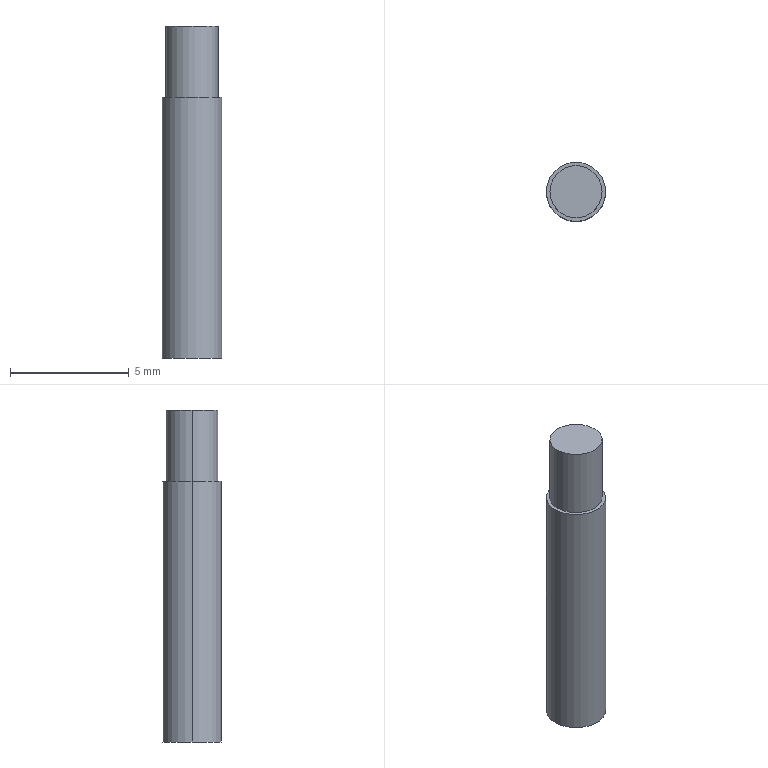Part | SolidWorks | features Extrusion 1, ICE 1 | 1 solid | 7 faces | box 2.5 x 2.5 x 14 mm | volume 65.4 mm3 | cylinder 4 | plane 3 | commonest cylinder face diameters 2.2 x2 2.5 x2
STEP:
#1=CARTESIAN_POINT('',(1.1,0.,14.));
#2=VERTEX_POINT('',#1);
#3=CARTESIAN_POINT('',(-1.1,0.,14.));
#4=VERTEX_POINT('',#3);
#5=CARTESIAN_POINT('',(0.,0.,14.));
#6=DIRECTION('',(0.,0.,1.));
#7=DIRECTION('',(1.,0.,0.));
#8=AXIS2_PLACEMENT_3D('',#5,#6,#7);
#9=CIRCLE('',#8,1.1);
#10=EDGE_CURVE('',#2,#4,#9,.T.);
#11=ORIENTED_EDGE('',*,*,#10,.F.);
#12=CARTESIAN_POINT('',(1.1,0.,11.));
#13=VERTEX_POINT('',#12);
#14=CARTESIAN_POINT('',(1.1,0.,14.));
#15=DIRECTION('',(0.,0.,-1.));
#16=VECTOR('',#15,1000.);
#17=LINE('',#14,#16);
#18=EDGE_CURVE('',#2,#13,#17,.T.);
#19=ORIENTED_EDGE('',*,*,#18,.T.);
#20=CARTESIAN_POINT('',(-1.1,0.,11.));
#21=VERTEX_POINT('',#20);
#22=CARTESIAN_POINT('',(0.,0.,11.));
#23=DIRECTION('',(0.,0.,1.));
#24=DIRECTION('',(1.,0.,0.));
#25=AXIS2_PLACEMENT_3D('',#22,#23,#24);
#26=CIRCLE('',#25,1.1);
#27=EDGE_CURVE('',#13,#21,#26,.T.);
#28=ORIENTED_EDGE('',*,*,#27,.T.);
#29=CARTESIAN_POINT('',(-1.1,0.,14.));
#30=DIRECTION('',(0.,0.,-1.));
#31=VECTOR('',#30,1000.);
#32=LINE('',#29,#31);
#33=EDGE_CURVE('',#4,#21,#32,.T.);
#34=ORIENTED_EDGE('',*,*,#33,.F.);
#35=EDGE_LOOP('',(#11,#19,#28,#34));
#36=FACE_OUTER_BOUND('',#35,.T.);
#37=CARTESIAN_POINT('',(0.,0.,14.));
#38=DIRECTION('',(0.,0.,-1.));
#39=DIRECTION('',(-1.,0.,0.));
#40=AXIS2_PLACEMENT_3D('',#37,#38,#39);
#41=CYLINDRICAL_SURFACE('',#40,1.1);
#42=ADVANCED_FACE('',(#36),#41,.T.);
#43=CARTESIAN_POINT('',(1.25,0.,11.));
#44=VERTEX_POINT('',#43);
#45=CARTESIAN_POINT('',(-1.25,0.,11.));
#46=VERTEX_POINT('',#45);
#47=CARTESIAN_POINT('',(0.,0.,11.));
#48=DIRECTION('',(0.,0.,1.));
#49=DIRECTION('',(1.,0.,0.));
#50=AXIS2_PLACEMENT_3D('',#47,#48,#49);
#51=CIRCLE('',#50,1.25);
#52=EDGE_CURVE('',#44,#46,#51,.T.);
#53=ORIENTED_EDGE('',*,*,#52,.F.);
#54=CARTESIAN_POINT('',(1.25,0.,0.));
#55=VERTEX_POINT('',#54);
#56=CARTESIAN_POINT('',(1.25,0.,11.));
#57=DIRECTION('',(0.,0.,-1.));
#58=VECTOR('',#57,1000.);
#59=LINE('',#56,#58);
#60=EDGE_CURVE('',#44,#55,#59,.T.);
#61=ORIENTED_EDGE('',*,*,#60,.T.);
#62=CARTESIAN_POINT('',(-1.25,0.,0.));
#63=VERTEX_POINT('',#62);
#64=CARTESIAN_POINT('',(0.,0.,0.));
#65=DIRECTION('',(0.,0.,1.));
#66=DIRECTION('',(1.,0.,0.));
#67=AXIS2_PLACEMENT_3D('',#64,#65,#66);
#68=CIRCLE('',#67,1.25);
#69=EDGE_CURVE('',#55,#63,#68,.T.);
#70=ORIENTED_EDGE('',*,*,#69,.T.);
#71=CARTESIAN_POINT('',(-1.25,0.,11.));
#72=DIRECTION('',(0.,0.,-1.));
#73=VECTOR('',#72,1000.);
#74=LINE('',#71,#73);
#75=EDGE_CURVE('',#46,#63,#74,.T.);
#76=ORIENTED_EDGE('',*,*,#75,.F.);
#77=EDGE_LOOP('',(#53,#61,#70,#76));
#78=FACE_OUTER_BOUND('',#77,.T.);
#79=CARTESIAN_POINT('',(0.,0.,11.));
#80=DIRECTION('',(0.,0.,-1.));
#81=DIRECTION('',(-1.,0.,0.));
#82=AXIS2_PLACEMENT_3D('',#79,#80,#81);
#83=CYLINDRICAL_SURFACE('',#82,1.25);
#84=ADVANCED_FACE('',(#78),#83,.T.);
#85=ORIENTED_EDGE('',*,*,#60,.F.);
#86=CARTESIAN_POINT('',(0.,0.,11.));
#87=DIRECTION('',(0.,0.,1.));
#88=DIRECTION('',(1.,0.,0.));
#89=AXIS2_PLACEMENT_3D('',#86,#87,#88);
#90=CIRCLE('',#89,1.25);
#91=EDGE_CURVE('',#46,#44,#90,.T.);
#92=ORIENTED_EDGE('',*,*,#91,.F.);
#93=ORIENTED_EDGE('',*,*,#75,.T.);
#94=CARTESIAN_POINT('',(0.,0.,0.));
#95=DIRECTION('',(0.,0.,1.));
#96=DIRECTION('',(1.,0.,0.));
#97=AXIS2_PLACEMENT_3D('',#94,#95,#96);
#98=CIRCLE('',#97,1.25);
#99=EDGE_CURVE('',#63,#55,#98,.T.);
#100=ORIENTED_EDGE('',*,*,#99,.T.);
#101=EDGE_LOOP('',(#85,#92,#93,#100));
#102=FACE_OUTER_BOUND('',#101,.T.);
#103=CARTESIAN_POINT('',(0.,0.,11.));
#104=DIRECTION('',(0.,0.,-1.));
#105=DIRECTION('',(-1.,0.,0.));
#106=AXIS2_PLACEMENT_3D('',#103,#104,#105);
#107=CYLINDRICAL_SURFACE('',#106,1.25);
#108=ADVANCED_FACE('',(#102),#107,.T.);
#109=CARTESIAN_POINT('',(0.,0.,11.));
#110=DIRECTION('',(0.,0.,1.));
#111=DIRECTION('',(1.,0.,0.));
#112=AXIS2_PLACEMENT_3D('',#109,#110,#111);
#113=CIRCLE('',#112,1.1);
#114=EDGE_CURVE('',#21,#13,#113,.T.);
#115=ORIENTED_EDGE('',*,*,#114,.F.);
#116=ORIENTED_EDGE('',*,*,#27,.F.);
#117=EDGE_LOOP('',(#115,#116));
#118=FACE_BOUND('',#117,.T.);
#119=ORIENTED_EDGE('',*,*,#91,.T.);
#120=ORIENTED_EDGE('',*,*,#52,.T.);
#121=EDGE_LOOP('',(#119,#120));
#122=FACE_OUTER_BOUND('',#121,.T.);
#123=CARTESIAN_POINT('',(0.,0.,11.));
#124=DIRECTION('',(0.,0.,1.));
#125=DIRECTION('',(1.,0.,0.));
#126=AXIS2_PLACEMENT_3D('',#123,#124,#125);
#127=PLANE('',#126);
#128=ADVANCED_FACE('',(#118,#122),#127,.T.);
#129=ORIENTED_EDGE('',*,*,#99,.F.);
#130=ORIENTED_EDGE('',*,*,#69,.F.);
#131=EDGE_LOOP('',(#129,#130));
#132=FACE_OUTER_BOUND('',#131,.T.);
#133=CARTESIAN_POINT('',(0.,0.,0.));
#134=DIRECTION('',(0.,0.,1.));
#135=DIRECTION('',(1.,0.,0.));
#136=AXIS2_PLACEMENT_3D('',#133,#134,#135);
#137=PLANE('',#136);
#138=ADVANCED_FACE('',(#132),#137,.F.);
#139=ORIENTED_EDGE('',*,*,#18,.F.);
#140=CARTESIAN_POINT('',(0.,0.,14.));
#141=DIRECTION('',(0.,0.,1.));
#142=DIRECTION('',(1.,0.,0.));
#143=AXIS2_PLACEMENT_3D('',#140,#141,#142);
#144=CIRCLE('',#143,1.1);
#145=EDGE_CURVE('',#4,#2,#144,.T.);
#146=ORIENTED_EDGE('',*,*,#145,.F.);
#147=ORIENTED_EDGE('',*,*,#33,.T.);
#148=ORIENTED_EDGE('',*,*,#114,.T.);
#149=EDGE_LOOP('',(#139,#146,#147,#148));
#150=FACE_OUTER_BOUND('',#149,.T.);
#151=CARTESIAN_POINT('',(0.,0.,14.));
#152=DIRECTION('',(0.,0.,-1.));
#153=DIRECTION('',(-1.,0.,0.));
#154=AXIS2_PLACEMENT_3D('',#151,#152,#153);
#155=CYLINDRICAL_SURFACE('',#154,1.1);
#156=ADVANCED_FACE('',(#150),#155,.T.);
#157=ORIENTED_EDGE('',*,*,#145,.T.);
#158=ORIENTED_EDGE('',*,*,#10,.T.);
#159=EDGE_LOOP('',(#157,#158));
#160=FACE_OUTER_BOUND('',#159,.T.);
#161=CARTESIAN_POINT('',(0.,0.,14.));
#162=DIRECTION('',(0.,0.,1.));
#163=DIRECTION('',(1.,0.,0.));
#164=AXIS2_PLACEMENT_3D('',#161,#162,#163);
#165=PLANE('',#164);
#166=ADVANCED_FACE('',(#160),#165,.T.);
#167=CLOSED_SHELL('',(#42,#84,#108,#128,#138,#156,#166));
#168=MANIFOLD_SOLID_BREP('',#167);
#169=CARTESIAN_POINT('',(0.,0.,0.));
#170=DIRECTION('',(0.,0.,1.));
#171=DIRECTION('',(1.,0.,0.));
#172=AXIS2_PLACEMENT_3D('',#169,#170,#171);
#173=(LENGTH_UNIT()NAMED_UNIT(*)SI_UNIT(.MILLI.,.METRE.));
#174=UNCERTAINTY_MEASURE_WITH_UNIT(LENGTH_MEASURE(0.00001),#173,'','');
#175=(NAMED_UNIT(*)PLANE_ANGLE_UNIT()SI_UNIT($,.RADIAN.));
#176=(NAMED_UNIT(*)SI_UNIT($,.STERADIAN.)SOLID_ANGLE_UNIT());
#177=(GEOMETRIC_REPRESENTATION_CONTEXT(3)GLOBAL_UNCERTAINTY_ASSIGNED_CONTEXT((#174))GLOBAL_UNIT_ASSIGNED_CONTEXT((#173,#175,#176))REPRESENTATION_CONTEXT('',''));
#178=ADVANCED_BREP_SHAPE_REPRESENTATION('',(#168,#172),#177);